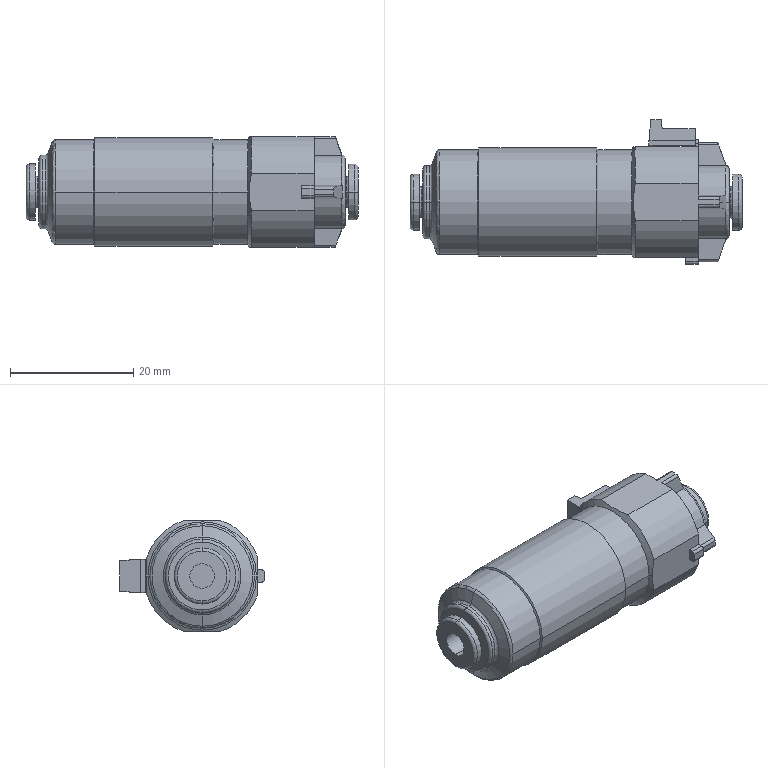Part | STEP file | 1 solid | 112 faces | box 53.9 x 23.5 x 18 mm | volume 11445 mm3 | plane 45 | cylinder 40 | torus 16 | cone 11 | commonest cylinder face diameters 0.8 x10 12 x6 4 x4 5 x4 9.1 x4 17 x4